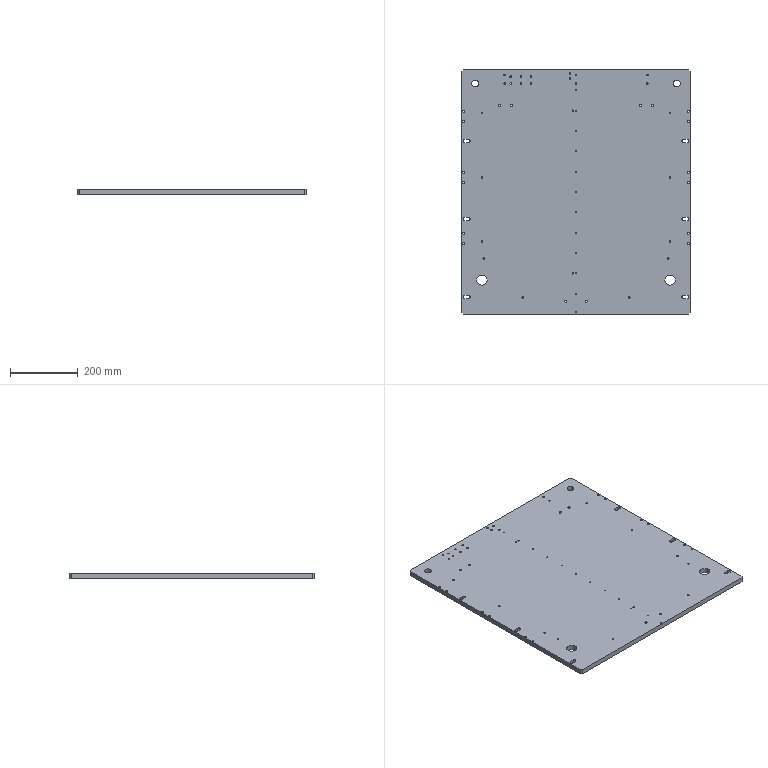CAM job | NX | 3-axis milling, drilling | part box 675 x 720 x 15 mm | stock box 675 x 720 x 15 mm
Tools:
number,name,description,diameter,corner_radius,flute_length,length,flutes
6,D6,平底铣刀-粗,6.0,0.0,25.0,75.0,2
9,D10,平底铣刀-粗,10.0,0.0,35.0,75.0,2
7,D6-J,平底铣刀-精,6.0,0.0,25.0,75.0,2
10,D10-J,平底铣刀-精,10.0,0.0,35.0,75.0,2
2,D6倒角刀,倒角刀,6.0,0.0,3.0,25.0,2
21,M4X0.7,丝锥,3.3,0.0,35.0,50.0,2
23,M6X1.0,丝锥,5.0,0.0,35.0,50.0,2
22,M8X1.25,丝锥,6.8,0.0,35.0,50.0,2
18,D4铰刀,Drilling Tool,4.0,0.0,75.0,100.0,6
1,C6定点钻,倒角刀,6.0,0.0,3.0,3.0,2
13,ZT3.4,钻头,3.4,0.0,35.0,50.0,2
15,ZT5.1,钻头,5.1,0.0,35.0,50.0,2
19,ZT10,钻头,10.0,0.0,35.0,50.0,2
17,ZT3.9,Drilling Tool,3.9,0.0,35.0,50.0,2
16,ZT6.9,Drilling Tool,6.9,0.0,35.0,50.0,2
Operations:
program,operation,operation_type,tool,method,geometry_group,spindle_rpm,surface_speed,feed_per_tooth,feed_cut,feed_plunge,cut_length_mm,path_length_mm,cut_time_min,machine_time_min
B,钻倒角_3,Operation,D6倒角刀,METHOD,W-B,2000.0,0.0,0.025,100.0,0.0,57.2,845.149,0.572,0.6508
B,钻倒角_4,Operation,D6倒角刀,METHOD,W-B,2000.0,0.0,0.025,100.0,0.0,10.6,604.209,0.106,0.1654
B,铣倒角_3,PlanarMilling,D6倒角刀,METHOD,W-B,4000.0,75.398,0.0375,300.0,100.0,666.753,6947.974,2.223,2.851
B,铣倒角_4,PlanarMilling,D6倒角刀,METHOD,W-B,4000.0,75.398,0.0375,300.0,100.0,143.492,1874.408,0.4783,0.6514
B,平面去毛刺6X45L_COPY_1,SurfaceContour,D6倒角刀,爬面_倒角-切深0-步距G,W-B,3500.0,65.972,0.1429,1000.0,100.0,2772.762,14445.651,2.773,3.94
A,选线往复层切开粗-中_COPY,PlanarMilling,D10,分层开粗-切深K-步距G,W-A,3000.0,94.245,0.3333,2000.0,100.0,7521.32,10144.314,3.761,4.023
A,打点-深0.8,Operation,C6定点钻,NONE,W-A,3000.0,56.0,0.01,60.0,90.0,108.0,3769.245,1.8,2.166
A,通孔-M4螺纹底孔,Operation,ZT3.4,NONE,W-A,1500.0,15.551,0.02,60.0,90.0,242.0,1154.083,4.033,4.125
A,通孔-精孔4.0预钻,Operation,ZT3.9,NONE,W-A,1500.0,18.378,0.0167,50.0,90.0,40.252,621.504,0.805,0.8632
A,通孔-M6螺纹底孔,Operation,ZT5.1,NONE,W-A,800.0,12.566,0.0625,100.0,90.0,851.0,4293.809,8.51,8.854
A,通孔-M8螺纹底孔,Operation,ZT6.9,NONE,W-A,600.0,12.818,0.1,120.0,90.0,144.0,1473.258,1.2,1.333
A,通孔-精孔12.0预钻,Operation,ZT10,NONE,W-A,500.0,31.102,0.12,120.0,90.0,41.009,738.018,0.3417,0.4114
A,通孔-精孔12.0预钻_2,Operation,ZT10,NONE,W-A,500.0,46.81,0.12,120.0,90.0,40.009,696.018,0.3334,0.399
A,通腰槽粗_1,VolumeBased25DMillingOperation,D6,METHOD,W-A,3500.0,65.973,0.1714,1200.0,100.0,20328.108,22689.71,16.94,17.176
A,铣孔开粗D8_1,CylinderMilling,D10,NONE,W-A,4000.0,100.531,0.1875,1500.0,100.0,4066.229,4931.229,2.711,2.797
A,铣孔开粗D8_2,CylinderMilling,D10,NONE,W-A,4000.0,100.531,0.1875,1500.0,100.0,9867.918,10691.918,6.579,6.661
A,钻倒角_1,Operation,D6倒角刀,METHOD,W-A,4000.0,75.398,0.01,80.0,0.0,57.2,805.149,0.715,0.7898
A,钻倒角_2,Operation,D6倒角刀,METHOD,W-A,4000.0,75.398,0.01,80.0,0.0,10.6,564.209,0.1325,0.1879
A,铣倒角_1,PlanarMilling,D6倒角刀,METHOD,W-A,4000.0,75.398,0.0375,300.0,100.0,737.712,7719.712,2.459,3.157
A,铣倒角_2,PlanarMilling,D6倒角刀,METHOD,W-A,4000.0,75.398,0.0625,500.0,100.0,140.862,1996.261,0.2817,0.4673
A,平面去毛刺6X45L_COPY,SurfaceContour,D6倒角刀,爬面_倒角-切深0-步距G,W-A,3500.0,65.972,0.1429,1000.0,100.0,2771.9,15423.788,2.772,4.037
A,腰槽精_1,VolumeBased25DMillingOperation,D6-J,METHOD,W-A,3700.0,32.0,0.0676,500.0,100.0,629.235,3216.13,1.258,1.517
A,底壁铣精光侧面-中_COPY,VolumeBased25DMillingOperation,D10-J,侧刃精光-切深K-步距G,W-A,3000.0,94.245,0.1333,800.0,100.0,286.444,953.12,0.3581,0.4247
A,铰孔,Operation,D4铰刀,METHOD,W-A,500.0,6.283,0.0167,50.0,0.0,34.0,609.001,0.68,0.7375
A,通孔-攻牙M4,Operation,M4X0.7,METHOD,W-A,500.0,5.184,0.0007,0.7,90.0,214.5,1099.083,306.429,306.517
A,通孔-攻牙M6,Operation,M6X1.0,METHOD,W-A,400.0,6.283,0.0013,1.0,90.0,721.5,4034.809,721.5,721.831
A,通孔-攻牙M8,Operation,M8X1.25,METHOD,W-A,300.0,6.409,0.0021,1.25,90.0,123.0,1431.258,98.4,98.531
A,底壁铣精光侧面-中_COPY_1,VolumeBased25DMillingOperation,D10-J,侧刃精光-切深K-步距G,W-A,3000.0,94.248,0.1,600.0,100.0,162.658,856.226,0.2711,0.3405
A,平面铣精光侧面-中-直线_COPY,PlanarMilling,D10-J,侧刃精光-切深K-步距G,W-A,3000.0,94.245,0.1333,800.0,100.0,168.569,3408.61,0.2107,0.5347